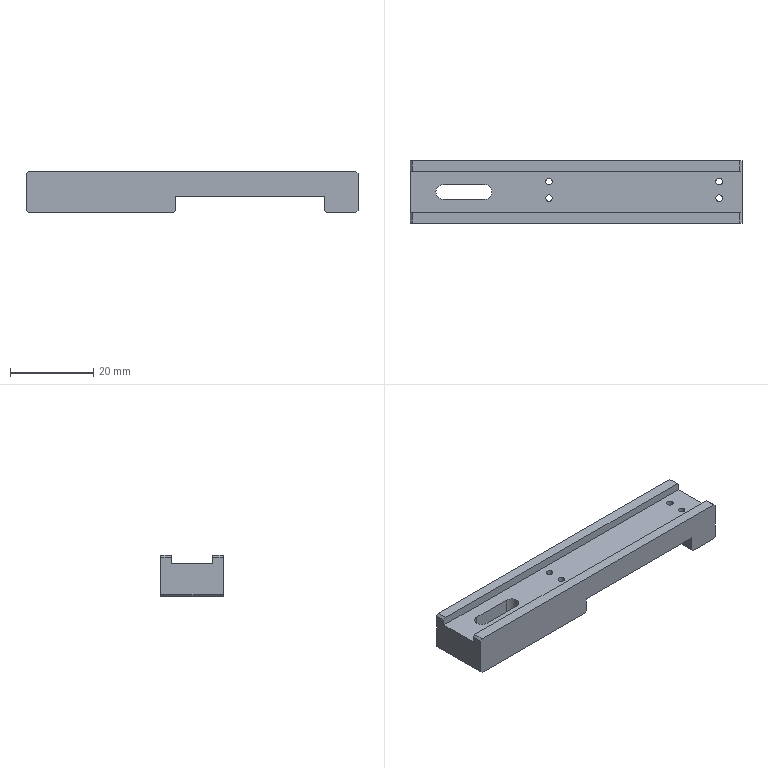NC program | NX | posted with a generic post | part box 80 x 15 x 10 mm
Whole program:
N10 G17 G21 G94 G90
(FLOOR_WALL_1_COPY_COPY , TOOL : D10JING)
N12 T14 M6
N14 G54
N16 G17 G0 G90 X26.497 Y15.5 S7500 M3
N18 G43 Z30. H14
N20 Z-1.
N22 G94 G1 Z-4. F1000.
N24 Y12.5
N26 Y-12.5 F1200.
N28 X21.498
N30 Y12.5
N32 X16.498
N34 Y-12.5
N36 X11.499
N38 Y12.5
N40 X6.499
N42 Y-12.5
N44 X1.5
N46 Y12.5
N48 Y15.5
N50 Z-1.
N52 G0 Z30.
N54 X1.
N56 Z-1.
N58 G1 Z-4. F1000.
N60 Y12.5
N62 Y-12.5 F1200.
N64 Y-15.5
N66 Z-1.
N68 G0 Z30.
N70 X27.
N72 Z-1.
N74 G1 Z-4. F1000.
N76 Y-12.5
N78 Y12.5 F1200.
N80 Y15.5
N82 Z-1.
N84 G0 Z30.
N86 M5
(PLANAR_MILL , TOOL : D6A45)
N88 T01 M6
N90 G54
N92 G17 G0 G90 X-27.766 Y-0.493 S7500 M3
N94 G43 Z30. H1
N96 Z1.
N98 G94 G1 Z-1. F1250.
N100 G3 X-27. Y-0.85 R1.
N102 G1 X-22.
N104 G3 X-21.15 Y0. R0.85
N106 X-22. Y0.85 R0.85
N108 G1 X-32.
N110 G3 X-32.85 Y0. R0.85
N112 X-32. Y-0.85 R0.85
N114 G1 X-27.
N116 G3 X-26.234 Y-0.493 R1.
N118 G1 Z1.
N120 G0 Z30.
N122 X-22.766 Y8.757
N124 Z1.
N126 G1 Z-1.
N128 G3 X-22. Y8.4 R1.
N130 G1 X-4.
N132 G2 X-3.1 Y7.5 R0.9
N134 G1 Y-7.5
N136 G2 X-4. Y-8.4 R0.9
N138 G1 X-40.
N140 G2 X-40.9 Y-7.5 R0.9
N142 G1 Y7.5
N144 G2 X-40. Y8.4 R0.9
N146 G1 X-22.
N148 G3 X-21.234 Y8.757 R1.
N150 G1 Z1.
N152 G0 Z30.
N154 X41.257 Y0.766
N156 Z1.
N158 G1 Z-1.
N160 G3 X40.9 Y0. R1.
N162 G1 Y-7.5
N164 G2 X40. Y-8.4 R0.9
N166 G1 X32.
N168 G2 X31.1 Y-7.5 R0.9
N170 G1 Y7.5
N172 G2 X32. Y8.4 R0.9
N174 G1 X40.
N176 G2 X40.9 Y7.5 R0.9
N178 G1 Y0.
N180 G3 X41.257 Y-0.766 R1.
N182 G1 Z1.
N184 G0 Z30.
(PLANAR_MILL_COPY , TOOL : D6A45)
N186 X0.022 Y9.932
N188 Z-3.
N190 G1 Z-5.
N192 X-0.469 Y9.232
N194 G3 X-0.618 Y8.4 R1.
N196 G1 X28.618
N198 G3 X28.469 Y9.232 R1.
N200 G1 X27.978 Y9.932
N202 Z-3.
N204 G0 Z30.
N206 Y-9.932
N208 Z-3.
N210 G1 Z-5.
N212 X28.469 Y-9.232
N214 G3 X28.618 Y-8.4 R1.
N216 G1 X-0.618
N218 G3 X-0.469 Y-9.232 R1.
N220 G1 X0.022 Y-9.932
N222 Z-3.
N224 G0 Z30.
N226 M5
N228 M2